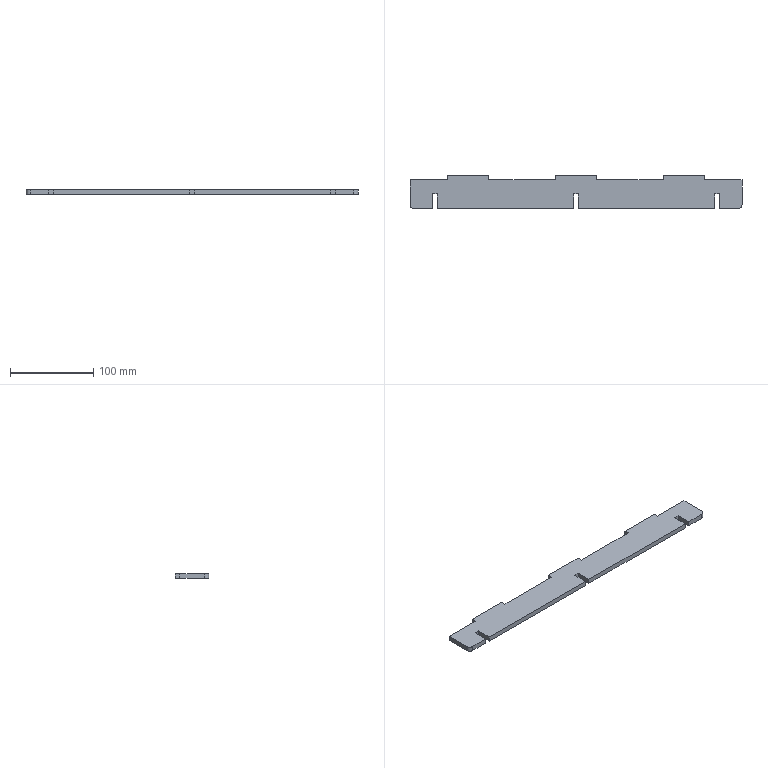Part | SolidWorks | features FlatPattern 1, SMBaseFlange 1, SheetMetal 1 | 1 solid | 32 faces | box 400 x 40.5 x 6 mm | volume 86942 mm3 | plane 30 | cylinder 2 | commonest cylinder face diameters 10 x2
STEP:
#1=CARTESIAN_POINT('',(-205.837,-343.504,0.));
#2=VERTEX_POINT('',#1);
#3=CARTESIAN_POINT('',(-205.837,-373.504,0.));
#4=VERTEX_POINT('',#3);
#5=CARTESIAN_POINT('',(-205.837,-343.504,0.));
#6=DIRECTION('',(0.,-1.,0.));
#7=VECTOR('',#6,1000.);
#8=LINE('',#5,#7);
#9=EDGE_CURVE('',#2,#4,#8,.T.);
#10=ORIENTED_EDGE('',*,*,#9,.F.);
#11=CARTESIAN_POINT('',(-205.837,-343.504,-6.));
#12=VERTEX_POINT('',#11);
#13=CARTESIAN_POINT('',(-205.837,-343.504,-6.));
#14=DIRECTION('',(0.,0.,1.));
#15=VECTOR('',#14,1000.);
#16=LINE('',#13,#15);
#17=EDGE_CURVE('',#12,#2,#16,.T.);
#18=ORIENTED_EDGE('',*,*,#17,.F.);
#19=CARTESIAN_POINT('',(-205.837,-373.504,-6.));
#20=VERTEX_POINT('',#19);
#21=CARTESIAN_POINT('',(-205.837,-343.504,-6.));
#22=DIRECTION('',(0.,-1.,0.));
#23=VECTOR('',#22,1000.);
#24=LINE('',#21,#23);
#25=EDGE_CURVE('',#12,#20,#24,.T.);
#26=ORIENTED_EDGE('',*,*,#25,.T.);
#27=CARTESIAN_POINT('',(-205.837,-373.504,-6.));
#28=DIRECTION('',(0.,0.,1.));
#29=VECTOR('',#28,1000.);
#30=LINE('',#27,#29);
#31=EDGE_CURVE('',#20,#4,#30,.T.);
#32=ORIENTED_EDGE('',*,*,#31,.T.);
#33=EDGE_LOOP('',(#10,#18,#26,#32));
#34=FACE_OUTER_BOUND('',#33,.T.);
#35=CARTESIAN_POINT('',(-205.837,-343.504,-6.));
#36=DIRECTION('',(-1.,0.,0.));
#37=DIRECTION('',(0.,0.,1.));
#38=AXIS2_PLACEMENT_3D('',#35,#36,#37);
#39=PLANE('',#38);
#40=ADVANCED_FACE('',(#34),#39,.T.);
#41=CARTESIAN_POINT('',(-160.837,-343.504,0.));
#42=VERTEX_POINT('',#41);
#43=CARTESIAN_POINT('',(-205.837,-343.504,0.));
#44=DIRECTION('',(-1.,0.,0.));
#45=VECTOR('',#44,1000.);
#46=LINE('',#43,#45);
#47=EDGE_CURVE('',#42,#2,#46,.T.);
#48=ORIENTED_EDGE('',*,*,#47,.F.);
#49=CARTESIAN_POINT('',(-160.837,-343.504,-6.));
#50=VERTEX_POINT('',#49);
#51=CARTESIAN_POINT('',(-160.837,-343.504,-6.));
#52=DIRECTION('',(0.,0.,1.));
#53=VECTOR('',#52,1000.);
#54=LINE('',#51,#53);
#55=EDGE_CURVE('',#50,#42,#54,.T.);
#56=ORIENTED_EDGE('',*,*,#55,.F.);
#57=CARTESIAN_POINT('',(-205.837,-343.504,-6.));
#58=DIRECTION('',(-1.,0.,0.));
#59=VECTOR('',#58,1000.);
#60=LINE('',#57,#59);
#61=EDGE_CURVE('',#50,#12,#60,.T.);
#62=ORIENTED_EDGE('',*,*,#61,.T.);
#63=ORIENTED_EDGE('',*,*,#17,.T.);
#64=EDGE_LOOP('',(#48,#56,#62,#63));
#65=FACE_OUTER_BOUND('',#64,.T.);
#66=CARTESIAN_POINT('',(-205.837,-343.504,-6.));
#67=DIRECTION('',(0.,1.,0.));
#68=DIRECTION('',(0.,0.,1.));
#69=AXIS2_PLACEMENT_3D('',#66,#67,#68);
#70=PLANE('',#69);
#71=ADVANCED_FACE('',(#65),#70,.T.);
#72=CARTESIAN_POINT('',(-160.837,-338.004,0.));
#73=VERTEX_POINT('',#72);
#74=CARTESIAN_POINT('',(-160.837,-343.504,0.));
#75=DIRECTION('',(0.,-1.,0.));
#76=VECTOR('',#75,1000.);
#77=LINE('',#74,#76);
#78=EDGE_CURVE('',#73,#42,#77,.T.);
#79=ORIENTED_EDGE('',*,*,#78,.F.);
#80=CARTESIAN_POINT('',(-160.837,-338.004,-6.));
#81=VERTEX_POINT('',#80);
#82=CARTESIAN_POINT('',(-160.837,-338.004,-6.));
#83=DIRECTION('',(0.,0.,1.));
#84=VECTOR('',#83,1000.);
#85=LINE('',#82,#84);
#86=EDGE_CURVE('',#81,#73,#85,.T.);
#87=ORIENTED_EDGE('',*,*,#86,.F.);
#88=CARTESIAN_POINT('',(-160.837,-343.504,-6.));
#89=DIRECTION('',(0.,-1.,0.));
#90=VECTOR('',#89,1000.);
#91=LINE('',#88,#90);
#92=EDGE_CURVE('',#81,#50,#91,.T.);
#93=ORIENTED_EDGE('',*,*,#92,.T.);
#94=ORIENTED_EDGE('',*,*,#55,.T.);
#95=EDGE_LOOP('',(#79,#87,#93,#94));
#96=FACE_OUTER_BOUND('',#95,.T.);
#97=CARTESIAN_POINT('',(-160.837,-343.504,-6.));
#98=DIRECTION('',(-1.,0.,0.));
#99=DIRECTION('',(0.,-1.,0.));
#100=AXIS2_PLACEMENT_3D('',#97,#98,#99);
#101=PLANE('',#100);
#102=ADVANCED_FACE('',(#96),#101,.T.);
#103=CARTESIAN_POINT('',(-110.837,-338.004,0.));
#104=VERTEX_POINT('',#103);
#105=CARTESIAN_POINT('',(-160.837,-338.004,0.));
#106=DIRECTION('',(-1.,0.,0.));
#107=VECTOR('',#106,1000.);
#108=LINE('',#105,#107);
#109=EDGE_CURVE('',#104,#73,#108,.T.);
#110=ORIENTED_EDGE('',*,*,#109,.F.);
#111=CARTESIAN_POINT('',(-110.837,-338.004,-6.));
#112=VERTEX_POINT('',#111);
#113=CARTESIAN_POINT('',(-110.837,-338.004,-6.));
#114=DIRECTION('',(0.,0.,1.));
#115=VECTOR('',#114,1000.);
#116=LINE('',#113,#115);
#117=EDGE_CURVE('',#112,#104,#116,.T.);
#118=ORIENTED_EDGE('',*,*,#117,.F.);
#119=CARTESIAN_POINT('',(-160.837,-338.004,-6.));
#120=DIRECTION('',(-1.,0.,0.));
#121=VECTOR('',#120,1000.);
#122=LINE('',#119,#121);
#123=EDGE_CURVE('',#112,#81,#122,.T.);
#124=ORIENTED_EDGE('',*,*,#123,.T.);
#125=ORIENTED_EDGE('',*,*,#86,.T.);
#126=EDGE_LOOP('',(#110,#118,#124,#125));
#127=FACE_OUTER_BOUND('',#126,.T.);
#128=CARTESIAN_POINT('',(-160.837,-338.004,-6.));
#129=DIRECTION('',(0.,1.,0.));
#130=DIRECTION('',(0.,0.,1.));
#131=AXIS2_PLACEMENT_3D('',#128,#129,#130);
#132=PLANE('',#131);
#133=ADVANCED_FACE('',(#127),#132,.T.);
#134=CARTESIAN_POINT('',(-110.837,-343.504,0.));
#135=VERTEX_POINT('',#134);
#136=CARTESIAN_POINT('',(-110.837,-338.004,0.));
#137=DIRECTION('',(0.,1.,0.));
#138=VECTOR('',#137,1000.);
#139=LINE('',#136,#138);
#140=EDGE_CURVE('',#135,#104,#139,.T.);
#141=ORIENTED_EDGE('',*,*,#140,.F.);
#142=CARTESIAN_POINT('',(-110.837,-343.504,-6.));
#143=VERTEX_POINT('',#142);
#144=CARTESIAN_POINT('',(-110.837,-343.504,-6.));
#145=DIRECTION('',(0.,0.,1.));
#146=VECTOR('',#145,1000.);
#147=LINE('',#144,#146);
#148=EDGE_CURVE('',#143,#135,#147,.T.);
#149=ORIENTED_EDGE('',*,*,#148,.F.);
#150=CARTESIAN_POINT('',(-110.837,-338.004,-6.));
#151=DIRECTION('',(0.,1.,0.));
#152=VECTOR('',#151,1000.);
#153=LINE('',#150,#152);
#154=EDGE_CURVE('',#143,#112,#153,.T.);
#155=ORIENTED_EDGE('',*,*,#154,.T.);
#156=ORIENTED_EDGE('',*,*,#117,.T.);
#157=EDGE_LOOP('',(#141,#149,#155,#156));
#158=FACE_OUTER_BOUND('',#157,.T.);
#159=CARTESIAN_POINT('',(-110.837,-338.004,-6.));
#160=DIRECTION('',(1.,0.,0.));
#161=DIRECTION('',(0.,1.,0.));
#162=AXIS2_PLACEMENT_3D('',#159,#160,#161);
#163=PLANE('',#162);
#164=ADVANCED_FACE('',(#158),#163,.T.);
#165=CARTESIAN_POINT('',(-30.837,-343.504,0.));
#166=VERTEX_POINT('',#165);
#167=CARTESIAN_POINT('',(-110.837,-343.504,0.));
#168=DIRECTION('',(-1.,0.,0.));
#169=VECTOR('',#168,1000.);
#170=LINE('',#167,#169);
#171=EDGE_CURVE('',#166,#135,#170,.T.);
#172=ORIENTED_EDGE('',*,*,#171,.F.);
#173=CARTESIAN_POINT('',(-30.837,-343.504,-6.));
#174=VERTEX_POINT('',#173);
#175=CARTESIAN_POINT('',(-30.837,-343.504,-6.));
#176=DIRECTION('',(0.,0.,1.));
#177=VECTOR('',#176,1000.);
#178=LINE('',#175,#177);
#179=EDGE_CURVE('',#174,#166,#178,.T.);
#180=ORIENTED_EDGE('',*,*,#179,.F.);
#181=CARTESIAN_POINT('',(-110.837,-343.504,-6.));
#182=DIRECTION('',(-1.,0.,0.));
#183=VECTOR('',#182,1000.);
#184=LINE('',#181,#183);
#185=EDGE_CURVE('',#174,#143,#184,.T.);
#186=ORIENTED_EDGE('',*,*,#185,.T.);
#187=ORIENTED_EDGE('',*,*,#148,.T.);
#188=EDGE_LOOP('',(#172,#180,#186,#187));
#189=FACE_OUTER_BOUND('',#188,.T.);
#190=CARTESIAN_POINT('',(-110.837,-343.504,-6.));
#191=DIRECTION('',(0.,1.,0.));
#192=DIRECTION('',(0.,0.,1.));
#193=AXIS2_PLACEMENT_3D('',#190,#191,#192);
#194=PLANE('',#193);
#195=ADVANCED_FACE('',(#189),#194,.T.);
#196=CARTESIAN_POINT('',(-30.837,-338.004,0.));
#197=VERTEX_POINT('',#196);
#198=CARTESIAN_POINT('',(-30.837,-338.004,0.));
#199=DIRECTION('',(0.,-1.,0.));
#200=VECTOR('',#199,1000.);
#201=LINE('',#198,#200);
#202=EDGE_CURVE('',#197,#166,#201,.T.);
#203=ORIENTED_EDGE('',*,*,#202,.F.);
#204=CARTESIAN_POINT('',(-30.837,-338.004,-6.));
#205=VERTEX_POINT('',#204);
#206=CARTESIAN_POINT('',(-30.837,-338.004,-6.));
#207=DIRECTION('',(0.,0.,1.));
#208=VECTOR('',#207,1000.);
#209=LINE('',#206,#208);
#210=EDGE_CURVE('',#205,#197,#209,.T.);
#211=ORIENTED_EDGE('',*,*,#210,.F.);
#212=CARTESIAN_POINT('',(-30.837,-338.004,-6.));
#213=DIRECTION('',(0.,-1.,0.));
#214=VECTOR('',#213,1000.);
#215=LINE('',#212,#214);
#216=EDGE_CURVE('',#205,#174,#215,.T.);
#217=ORIENTED_EDGE('',*,*,#216,.T.);
#218=ORIENTED_EDGE('',*,*,#179,.T.);
#219=EDGE_LOOP('',(#203,#211,#217,#218));
#220=FACE_OUTER_BOUND('',#219,.T.);
#221=CARTESIAN_POINT('',(-30.837,-338.004,-6.));
#222=DIRECTION('',(-1.,0.,0.));
#223=DIRECTION('',(0.,-1.,0.));
#224=AXIS2_PLACEMENT_3D('',#221,#222,#223);
#225=PLANE('',#224);
#226=ADVANCED_FACE('',(#220),#225,.T.);
#227=CARTESIAN_POINT('',(19.163,-338.004,0.));
#228=VERTEX_POINT('',#227);
#229=CARTESIAN_POINT('',(19.163,-338.004,0.));
#230=DIRECTION('',(-1.,0.,0.));
#231=VECTOR('',#230,1000.);
#232=LINE('',#229,#231);
#233=EDGE_CURVE('',#228,#197,#232,.T.);
#234=ORIENTED_EDGE('',*,*,#233,.F.);
#235=CARTESIAN_POINT('',(19.163,-338.004,-6.));
#236=VERTEX_POINT('',#235);
#237=CARTESIAN_POINT('',(19.163,-338.004,-6.));
#238=DIRECTION('',(0.,0.,1.));
#239=VECTOR('',#238,1000.);
#240=LINE('',#237,#239);
#241=EDGE_CURVE('',#236,#228,#240,.T.);
#242=ORIENTED_EDGE('',*,*,#241,.F.);
#243=CARTESIAN_POINT('',(19.163,-338.004,-6.));
#244=DIRECTION('',(-1.,0.,0.));
#245=VECTOR('',#244,1000.);
#246=LINE('',#243,#245);
#247=EDGE_CURVE('',#236,#205,#246,.T.);
#248=ORIENTED_EDGE('',*,*,#247,.T.);
#249=ORIENTED_EDGE('',*,*,#210,.T.);
#250=EDGE_LOOP('',(#234,#242,#248,#249));
#251=FACE_OUTER_BOUND('',#250,.T.);
#252=CARTESIAN_POINT('',(19.163,-338.004,-6.));
#253=DIRECTION('',(0.,1.,0.));
#254=DIRECTION('',(0.,0.,1.));
#255=AXIS2_PLACEMENT_3D('',#252,#253,#254);
#256=PLANE('',#255);
#257=ADVANCED_FACE('',(#251),#256,.T.);
#258=CARTESIAN_POINT('',(19.163,-343.504,0.));
#259=VERTEX_POINT('',#258);
#260=CARTESIAN_POINT('',(19.163,-343.504,0.));
#261=DIRECTION('',(0.,1.,0.));
#262=VECTOR('',#261,1000.);
#263=LINE('',#260,#262);
#264=EDGE_CURVE('',#259,#228,#263,.T.);
#265=ORIENTED_EDGE('',*,*,#264,.F.);
#266=CARTESIAN_POINT('',(19.163,-343.504,-6.));
#267=VERTEX_POINT('',#266);
#268=CARTESIAN_POINT('',(19.163,-343.504,-6.));
#269=DIRECTION('',(0.,0.,1.));
#270=VECTOR('',#269,1000.);
#271=LINE('',#268,#270);
#272=EDGE_CURVE('',#267,#259,#271,.T.);
#273=ORIENTED_EDGE('',*,*,#272,.F.);
#274=CARTESIAN_POINT('',(19.163,-343.504,-6.));
#275=DIRECTION('',(0.,1.,0.));
#276=VECTOR('',#275,1000.);
#277=LINE('',#274,#276);
#278=EDGE_CURVE('',#267,#236,#277,.T.);
#279=ORIENTED_EDGE('',*,*,#278,.T.);
#280=ORIENTED_EDGE('',*,*,#241,.T.);
#281=EDGE_LOOP('',(#265,#273,#279,#280));
#282=FACE_OUTER_BOUND('',#281,.T.);
#283=CARTESIAN_POINT('',(19.163,-343.504,-6.));
#284=DIRECTION('',(1.,0.,0.));
#285=DIRECTION('',(0.,1.,0.));
#286=AXIS2_PLACEMENT_3D('',#283,#284,#285);
#287=PLANE('',#286);
#288=ADVANCED_FACE('',(#282),#287,.T.);
#289=CARTESIAN_POINT('',(99.163,-343.504,0.));
#290=VERTEX_POINT('',#289);
#291=CARTESIAN_POINT('',(19.163,-343.504,0.));
#292=DIRECTION('',(-1.,0.,0.));
#293=VECTOR('',#292,1000.);
#294=LINE('',#291,#293);
#295=EDGE_CURVE('',#290,#259,#294,.T.);
#296=ORIENTED_EDGE('',*,*,#295,.F.);
#297=CARTESIAN_POINT('',(99.163,-343.504,-6.));
#298=VERTEX_POINT('',#297);
#299=CARTESIAN_POINT('',(99.163,-343.504,-6.));
#300=DIRECTION('',(0.,0.,1.));
#301=VECTOR('',#300,1000.);
#302=LINE('',#299,#301);
#303=EDGE_CURVE('',#298,#290,#302,.T.);
#304=ORIENTED_EDGE('',*,*,#303,.F.);
#305=CARTESIAN_POINT('',(19.163,-343.504,-6.));
#306=DIRECTION('',(-1.,0.,0.));
#307=VECTOR('',#306,1000.);
#308=LINE('',#305,#307);
#309=EDGE_CURVE('',#298,#267,#308,.T.);
#310=ORIENTED_EDGE('',*,*,#309,.T.);
#311=ORIENTED_EDGE('',*,*,#272,.T.);
#312=EDGE_LOOP('',(#296,#304,#310,#311));
#313=FACE_OUTER_BOUND('',#312,.T.);
#314=CARTESIAN_POINT('',(19.163,-343.504,-6.));
#315=DIRECTION('',(0.,1.,0.));
#316=DIRECTION('',(0.,0.,1.));
#317=AXIS2_PLACEMENT_3D('',#314,#315,#316);
#318=PLANE('',#317);
#319=ADVANCED_FACE('',(#313),#318,.T.);
#320=CARTESIAN_POINT('',(99.163,-338.004,0.));
#321=VERTEX_POINT('',#320);
#322=CARTESIAN_POINT('',(99.163,-338.004,0.));
#323=DIRECTION('',(0.,-1.,0.));
#324=VECTOR('',#323,1000.);
#325=LINE('',#322,#324);
#326=EDGE_CURVE('',#321,#290,#325,.T.);
#327=ORIENTED_EDGE('',*,*,#326,.F.);
#328=CARTESIAN_POINT('',(99.163,-338.004,-6.));
#329=VERTEX_POINT('',#328);
#330=CARTESIAN_POINT('',(99.163,-338.004,-6.));
#331=DIRECTION('',(0.,0.,1.));
#332=VECTOR('',#331,1000.);
#333=LINE('',#330,#332);
#334=EDGE_CURVE('',#329,#321,#333,.T.);
#335=ORIENTED_EDGE('',*,*,#334,.F.);
#336=CARTESIAN_POINT('',(99.163,-338.004,-6.));
#337=DIRECTION('',(0.,-1.,0.));
#338=VECTOR('',#337,1000.);
#339=LINE('',#336,#338);
#340=EDGE_CURVE('',#329,#298,#339,.T.);
#341=ORIENTED_EDGE('',*,*,#340,.T.);
#342=ORIENTED_EDGE('',*,*,#303,.T.);
#343=EDGE_LOOP('',(#327,#335,#341,#342));
#344=FACE_OUTER_BOUND('',#343,.T.);
#345=CARTESIAN_POINT('',(99.163,-338.004,-6.));
#346=DIRECTION('',(-1.,0.,0.));
#347=DIRECTION('',(0.,0.,1.));
#348=AXIS2_PLACEMENT_3D('',#345,#346,#347);
#349=PLANE('',#348);
#350=ADVANCED_FACE('',(#344),#349,.T.);
#351=CARTESIAN_POINT('',(149.163,-338.004,0.));
#352=VERTEX_POINT('',#351);
#353=CARTESIAN_POINT('',(149.163,-338.004,0.));
#354=DIRECTION('',(-1.,0.,0.));
#355=VECTOR('',#354,1000.);
#356=LINE('',#353,#355);
#357=EDGE_CURVE('',#352,#321,#356,.T.);
#358=ORIENTED_EDGE('',*,*,#357,.F.);
#359=CARTESIAN_POINT('',(149.163,-338.004,-6.));
#360=VERTEX_POINT('',#359);
#361=CARTESIAN_POINT('',(149.163,-338.004,-6.));
#362=DIRECTION('',(0.,0.,1.));
#363=VECTOR('',#362,1000.);
#364=LINE('',#361,#363);
#365=EDGE_CURVE('',#360,#352,#364,.T.);
#366=ORIENTED_EDGE('',*,*,#365,.F.);
#367=CARTESIAN_POINT('',(149.163,-338.004,-6.));
#368=DIRECTION('',(-1.,0.,0.));
#369=VECTOR('',#368,1000.);
#370=LINE('',#367,#369);
#371=EDGE_CURVE('',#360,#329,#370,.T.);
#372=ORIENTED_EDGE('',*,*,#371,.T.);
#373=ORIENTED_EDGE('',*,*,#334,.T.);
#374=EDGE_LOOP('',(#358,#366,#372,#373));
#375=FACE_OUTER_BOUND('',#374,.T.);
#376=CARTESIAN_POINT('',(149.163,-338.004,-6.));
#377=DIRECTION('',(0.,1.,0.));
#378=DIRECTION('',(0.,0.,1.));
#379=AXIS2_PLACEMENT_3D('',#376,#377,#378);
#380=PLANE('',#379);
#381=ADVANCED_FACE('',(#375),#380,.T.);
#382=CARTESIAN_POINT('',(149.163,-343.504,0.));
#383=VERTEX_POINT('',#382);
#384=CARTESIAN_POINT('',(149.163,-343.504,0.));
#385=DIRECTION('',(0.,1.,0.));
#386=VECTOR('',#385,1000.);
#387=LINE('',#384,#386);
#388=EDGE_CURVE('',#383,#352,#387,.T.);
#389=ORIENTED_EDGE('',*,*,#388,.F.);
#390=CARTESIAN_POINT('',(149.163,-343.504,-6.));
#391=VERTEX_POINT('',#390);
#392=CARTESIAN_POINT('',(149.163,-343.504,-6.));
#393=DIRECTION('',(0.,0.,1.));
#394=VECTOR('',#393,1000.);
#395=LINE('',#392,#394);
#396=EDGE_CURVE('',#391,#383,#395,.T.);
#397=ORIENTED_EDGE('',*,*,#396,.F.);
#398=CARTESIAN_POINT('',(149.163,-343.504,-6.));
#399=DIRECTION('',(0.,1.,0.));
#400=VECTOR('',#399,1000.);
#401=LINE('',#398,#400);
#402=EDGE_CURVE('',#391,#360,#401,.T.);
#403=ORIENTED_EDGE('',*,*,#402,.T.);
#404=ORIENTED_EDGE('',*,*,#365,.T.);
#405=EDGE_LOOP('',(#389,#397,#403,#404));
#406=FACE_OUTER_BOUND('',#405,.T.);
#407=CARTESIAN_POINT('',(149.163,-343.504,-6.));
#408=DIRECTION('',(1.,0.,0.));
#409=DIRECTION('',(0.,0.,-1.));
#410=AXIS2_PLACEMENT_3D('',#407,#408,#409);
#411=PLANE('',#410);
#412=ADVANCED_FACE('',(#406),#411,.T.);
#413=CARTESIAN_POINT('',(194.163,-343.504,0.));
#414=VERTEX_POINT('',#413);
#415=CARTESIAN_POINT('',(149.163,-343.504,0.));
#416=DIRECTION('',(-1.,0.,0.));
#417=VECTOR('',#416,1000.);
#418=LINE('',#415,#417);
#419=EDGE_CURVE('',#414,#383,#418,.T.);
#420=ORIENTED_EDGE('',*,*,#419,.F.);
#421=CARTESIAN_POINT('',(194.163,-343.504,-6.));
#422=VERTEX_POINT('',#421);
#423=CARTESIAN_POINT('',(194.163,-343.504,-6.));
#424=DIRECTION('',(0.,0.,1.));
#425=VECTOR('',#424,1000.);
#426=LINE('',#423,#425);
#427=EDGE_CURVE('',#422,#414,#426,.T.);
#428=ORIENTED_EDGE('',*,*,#427,.F.);
#429=CARTESIAN_POINT('',(149.163,-343.504,-6.));
#430=DIRECTION('',(-1.,0.,0.));
#431=VECTOR('',#430,1000.);
#432=LINE('',#429,#431);
#433=EDGE_CURVE('',#422,#391,#432,.T.);
#434=ORIENTED_EDGE('',*,*,#433,.T.);
#435=ORIENTED_EDGE('',*,*,#396,.T.);
#436=EDGE_LOOP('',(#420,#428,#434,#435));
#437=FACE_OUTER_BOUND('',#436,.T.);
#438=CARTESIAN_POINT('',(149.163,-343.504,-6.));
#439=DIRECTION('',(0.,1.,0.));
#440=DIRECTION('',(0.,0.,1.));
#441=AXIS2_PLACEMENT_3D('',#438,#439,#440);
#442=PLANE('',#441);
#443=ADVANCED_FACE('',(#437),#442,.T.);
#444=CARTESIAN_POINT('',(194.163,-373.504,0.));
#445=VERTEX_POINT('',#444);
#446=CARTESIAN_POINT('',(194.163,-343.504,0.));
#447=DIRECTION('',(0.,1.,0.));
#448=VECTOR('',#447,1000.);
#449=LINE('',#446,#448);
#450=EDGE_CURVE('',#445,#414,#449,.T.);
#451=ORIENTED_EDGE('',*,*,#450,.F.);
#452=CARTESIAN_POINT('',(194.163,-373.504,-6.));
#453=VERTEX_POINT('',#452);
#454=CARTESIAN_POINT('',(194.163,-373.504,-6.));
#455=DIRECTION('',(0.,0.,1.));
#456=VECTOR('',#455,1000.);
#457=LINE('',#454,#456);
#458=EDGE_CURVE('',#453,#445,#457,.T.);
#459=ORIENTED_EDGE('',*,*,#458,.F.);
#460=CARTESIAN_POINT('',(194.163,-343.504,-6.));
#461=DIRECTION('',(0.,1.,0.));
#462=VECTOR('',#461,1000.);
#463=LINE('',#460,#462);
#464=EDGE_CURVE('',#453,#422,#463,.T.);
#465=ORIENTED_EDGE('',*,*,#464,.T.);
#466=ORIENTED_EDGE('',*,*,#427,.T.);
#467=EDGE_LOOP('',(#451,#459,#465,#466));
#468=FACE_OUTER_BOUND('',#467,.T.);
#469=CARTESIAN_POINT('',(194.163,-343.504,-6.));
#470=DIRECTION('',(1.,0.,0.));
#471=DIRECTION('',(0.,0.,-1.));
#472=AXIS2_PLACEMENT_3D('',#469,#470,#471);
#473=PLANE('',#472);
#474=ADVANCED_FACE('',(#468),#473,.T.);
#475=CARTESIAN_POINT('',(189.163,-378.504,0.));
#476=VERTEX_POINT('',#475);
#477=CARTESIAN_POINT('',(189.163,-373.504,0.));
#478=DIRECTION('',(0.,0.,1.));
#479=DIRECTION('',(1.,0.,0.));
#480=AXIS2_PLACEMENT_3D('',#477,#478,#479);
#481=CIRCLE('',#480,5.);
#482=EDGE_CURVE('',#476,#445,#481,.T.);
#483=ORIENTED_EDGE('',*,*,#482,.F.);
#484=CARTESIAN_POINT('',(189.163,-378.504,-6.));
#485=VERTEX_POINT('',#484);
#486=CARTESIAN_POINT('',(189.163,-378.504,-6.));
#487=DIRECTION('',(0.,0.,1.));
#488=VECTOR('',#487,1000.);
#489=LINE('',#486,#488);
#490=EDGE_CURVE('',#485,#476,#489,.T.);
#491=ORIENTED_EDGE('',*,*,#490,.F.);
#492=CARTESIAN_POINT('',(189.163,-373.504,-6.));
#493=DIRECTION('',(0.,0.,1.));
#494=DIRECTION('',(1.,0.,0.));
#495=AXIS2_PLACEMENT_3D('',#492,#493,#494);
#496=CIRCLE('',#495,5.);
#497=EDGE_CURVE('',#485,#453,#496,.T.);
#498=ORIENTED_EDGE('',*,*,#497,.T.);
#499=ORIENTED_EDGE('',*,*,#458,.T.);
#500=EDGE_LOOP('',(#483,#491,#498,#499));
#501=FACE_OUTER_BOUND('',#500,.T.);
#502=CARTESIAN_POINT('',(189.163,-373.504,-6.));
#503=DIRECTION('',(0.,0.,1.));
#504=DIRECTION('',(1.,0.,0.));
#505=AXIS2_PLACEMENT_3D('',#502,#503,#504);
#506=CYLINDRICAL_SURFACE('',#505,5.);
#507=ADVANCED_FACE('',(#501),#506,.T.);
#508=CARTESIAN_POINT('',(167.163,-378.504,0.));
#509=VERTEX_POINT('',#508);
#510=CARTESIAN_POINT('',(167.163,-378.504,0.));
#511=DIRECTION('',(1.,0.,0.));
#512=VECTOR('',#511,1000.);
#513=LINE('',#510,#512);
#514=EDGE_CURVE('',#509,#476,#513,.T.);
#515=ORIENTED_EDGE('',*,*,#514,.F.);
#516=CARTESIAN_POINT('',(167.163,-378.504,-6.));
#517=VERTEX_POINT('',#516);
#518=CARTESIAN_POINT('',(167.163,-378.504,-6.));
#519=DIRECTION('',(0.,0.,1.));
#520=VECTOR('',#519,1000.);
#521=LINE('',#518,#520);
#522=EDGE_CURVE('',#517,#509,#521,.T.);
#523=ORIENTED_EDGE('',*,*,#522,.F.);
#524=CARTESIAN_POINT('',(167.163,-378.504,-6.));
#525=DIRECTION('',(1.,0.,0.));
#526=VECTOR('',#525,1000.);
#527=LINE('',#524,#526);
#528=EDGE_CURVE('',#517,#485,#527,.T.);
#529=ORIENTED_EDGE('',*,*,#528,.T.);
#530=ORIENTED_EDGE('',*,*,#490,.T.);
#531=EDGE_LOOP('',(#515,#523,#529,#530));
#532=FACE_OUTER_BOUND('',#531,.T.);
#533=CARTESIAN_POINT('',(167.163,-378.504,-6.));
#534=DIRECTION('',(0.,-1.,0.));
#535=DIRECTION('',(0.,0.,-1.));
#536=AXIS2_PLACEMENT_3D('',#533,#534,#535);
#537=PLANE('',#536);
#538=ADVANCED_FACE('',(#532),#537,.T.);
#539=CARTESIAN_POINT('',(167.163,-360.504,0.));
#540=VERTEX_POINT('',#539);
#541=CARTESIAN_POINT('',(167.163,-360.504,0.));
#542=DIRECTION('',(0.,-1.,0.));
#543=VECTOR('',#542,1000.);
#544=LINE('',#541,#543);
#545=EDGE_CURVE('',#540,#509,#544,.T.);
#546=ORIENTED_EDGE('',*,*,#545,.F.);
#547=CARTESIAN_POINT('',(167.163,-360.504,-6.));
#548=VERTEX_POINT('',#547);
#549=CARTESIAN_POINT('',(167.163,-360.504,-6.));
#550=DIRECTION('',(0.,0.,1.));
#551=VECTOR('',#550,1000.);
#552=LINE('',#549,#551);
#553=EDGE_CURVE('',#548,#540,#552,.T.);
#554=ORIENTED_EDGE('',*,*,#553,.F.);
#555=CARTESIAN_POINT('',(167.163,-360.504,-6.));
#556=DIRECTION('',(0.,-1.,0.));
#557=VECTOR('',#556,1000.);
#558=LINE('',#555,#557);
#559=EDGE_CURVE('',#548,#517,#558,.T.);
#560=ORIENTED_EDGE('',*,*,#559,.T.);
#561=ORIENTED_EDGE('',*,*,#522,.T.);
#562=EDGE_LOOP('',(#546,#554,#560,#561));
#563=FACE_OUTER_BOUND('',#562,.T.);
#564=CARTESIAN_POINT('',(167.163,-360.504,-6.));
#565=DIRECTION('',(-1.,0.,0.));
#566=DIRECTION('',(0.,0.,1.));
#567=AXIS2_PLACEMENT_3D('',#564,#565,#566);
#568=PLANE('',#567);
#569=ADVANCED_FACE('',(#563),#568,.T.);
#570=CARTESIAN_POINT('',(161.163,-360.504,0.));
#571=VERTEX_POINT('',#570);
#572=CARTESIAN_POINT('',(161.163,-360.504,0.));
#573=DIRECTION('',(1.,0.,0.));
#574=VECTOR('',#573,1000.);
#575=LINE('',#572,#574);
#576=EDGE_CURVE('',#571,#540,#575,.T.);
#577=ORIENTED_EDGE('',*,*,#576,.F.);
#578=CARTESIAN_POINT('',(161.163,-360.504,-6.));
#579=VERTEX_POINT('',#578);
#580=CARTESIAN_POINT('',(161.163,-360.504,-6.));
#581=DIRECTION('',(0.,0.,1.));
#582=VECTOR('',#581,1000.);
#583=LINE('',#580,#582);
#584=EDGE_CURVE('',#579,#571,#583,.T.);
#585=ORIENTED_EDGE('',*,*,#584,.F.);
#586=CARTESIAN_POINT('',(161.163,-360.504,-6.));
#587=DIRECTION('',(1.,0.,0.));
#588=VECTOR('',#587,1000.);
#589=LINE('',#586,#588);
#590=EDGE_CURVE('',#579,#548,#589,.T.);
#591=ORIENTED_EDGE('',*,*,#590,.T.);
#592=ORIENTED_EDGE('',*,*,#553,.T.);
#593=EDGE_LOOP('',(#577,#585,#591,#592));
#594=FACE_OUTER_BOUND('',#593,.T.);
#595=CARTESIAN_POINT('',(161.163,-360.504,-6.));
#596=DIRECTION('',(0.,-1.,0.));
#597=DIRECTION('',(0.,0.,-1.));
#598=AXIS2_PLACEMENT_3D('',#595,#596,#597);
#599=PLANE('',#598);
#600=ADVANCED_FACE('',(#594),#599,.T.);
#601=CARTESIAN_POINT('',(161.163,-378.504,0.));
#602=VERTEX_POINT('',#601);
#603=CARTESIAN_POINT('',(161.163,-378.504,0.));
#604=DIRECTION('',(0.,1.,0.));
#605=VECTOR('',#604,1000.);
#606=LINE('',#603,#605);
#607=EDGE_CURVE('',#602,#571,#606,.T.);
#608=ORIENTED_EDGE('',*,*,#607,.F.);
#609=CARTESIAN_POINT('',(161.163,-378.504,-6.));
#610=VERTEX_POINT('',#609);
#611=CARTESIAN_POINT('',(161.163,-378.504,-6.));
#612=DIRECTION('',(0.,0.,1.));
#613=VECTOR('',#612,1000.);
#614=LINE('',#611,#613);
#615=EDGE_CURVE('',#610,#602,#614,.T.);
#616=ORIENTED_EDGE('',*,*,#615,.F.);
#617=CARTESIAN_POINT('',(161.163,-378.504,-6.));
#618=DIRECTION('',(0.,1.,0.));
#619=VECTOR('',#618,1000.);
#620=LINE('',#617,#619);
#621=EDGE_CURVE('',#610,#579,#620,.T.);
#622=ORIENTED_EDGE('',*,*,#621,.T.);
#623=ORIENTED_EDGE('',*,*,#584,.T.);
#624=EDGE_LOOP('',(#608,#616,#622,#623));
#625=FACE_OUTER_BOUND('',#624,.T.);
#626=CARTESIAN_POINT('',(161.163,-378.504,-6.));
#627=DIRECTION('',(1.,0.,0.));
#628=DIRECTION('',(0.,0.,-1.));
#629=AXIS2_PLACEMENT_3D('',#626,#627,#628);
#630=PLANE('',#629);
#631=ADVANCED_FACE('',(#625),#630,.T.);
#632=CARTESIAN_POINT('',(-2.837,-378.504,0.));
#633=VERTEX_POINT('',#632);
#634=CARTESIAN_POINT('',(-2.837,-378.504,0.));
#635=DIRECTION('',(1.,0.,0.));
#636=VECTOR('',#635,1000.);
#637=LINE('',#634,#636);
#638=EDGE_CURVE('',#633,#602,#637,.T.);
#639=ORIENTED_EDGE('',*,*,#638,.F.);
#640=CARTESIAN_POINT('',(-2.837,-378.504,-6.));
#641=VERTEX_POINT('',#640);
#642=CARTESIAN_POINT('',(-2.837,-378.504,-6.));
#643=DIRECTION('',(0.,0.,1.));
#644=VECTOR('',#643,1000.);
#645=LINE('',#642,#644);
#646=EDGE_CURVE('',#641,#633,#645,.T.);
#647=ORIENTED_EDGE('',*,*,#646,.F.);
#648=CARTESIAN_POINT('',(-2.837,-378.504,-6.));
#649=DIRECTION('',(1.,0.,0.));
#650=VECTOR('',#649,1000.);
#651=LINE('',#648,#650);
#652=EDGE_CURVE('',#641,#610,#651,.T.);
#653=ORIENTED_EDGE('',*,*,#652,.T.);
#654=ORIENTED_EDGE('',*,*,#615,.T.);
#655=EDGE_LOOP('',(#639,#647,#653,#654));
#656=FACE_OUTER_BOUND('',#655,.T.);
#657=CARTESIAN_POINT('',(-2.837,-378.504,-6.));
#658=DIRECTION('',(0.,-1.,0.));
#659=DIRECTION('',(0.,0.,-1.));
#660=AXIS2_PLACEMENT_3D('',#657,#658,#659);
#661=PLANE('',#660);
#662=ADVANCED_FACE('',(#656),#661,.T.);
#663=CARTESIAN_POINT('',(-2.837,-360.504,0.));
#664=VERTEX_POINT('',#663);
#665=CARTESIAN_POINT('',(-2.837,-360.504,0.));
#666=DIRECTION('',(0.,-1.,0.));
#667=VECTOR('',#666,1000.);
#668=LINE('',#665,#667);
#669=EDGE_CURVE('',#664,#633,#668,.T.);
#670=ORIENTED_EDGE('',*,*,#669,.F.);
#671=CARTESIAN_POINT('',(-2.837,-360.504,-6.));
#672=VERTEX_POINT('',#671);
#673=CARTESIAN_POINT('',(-2.837,-360.504,-6.));
#674=DIRECTION('',(0.,0.,1.));
#675=VECTOR('',#674,1000.);
#676=LINE('',#673,#675);
#677=EDGE_CURVE('',#672,#664,#676,.T.);
#678=ORIENTED_EDGE('',*,*,#677,.F.);
#679=CARTESIAN_POINT('',(-2.837,-360.504,-6.));
#680=DIRECTION('',(0.,-1.,0.));
#681=VECTOR('',#680,1000.);
#682=LINE('',#679,#681);
#683=EDGE_CURVE('',#672,#641,#682,.T.);
#684=ORIENTED_EDGE('',*,*,#683,.T.);
#685=ORIENTED_EDGE('',*,*,#646,.T.);
#686=EDGE_LOOP('',(#670,#678,#684,#685));
#687=FACE_OUTER_BOUND('',#686,.T.);
#688=CARTESIAN_POINT('',(-2.837,-360.504,-6.));
#689=DIRECTION('',(-1.,0.,0.));
#690=DIRECTION('',(0.,0.,1.));
#691=AXIS2_PLACEMENT_3D('',#688,#689,#690);
#692=PLANE('',#691);
#693=ADVANCED_FACE('',(#687),#692,.T.);
#694=CARTESIAN_POINT('',(-8.837,-360.504,0.));
#695=VERTEX_POINT('',#694);
#696=CARTESIAN_POINT('',(-8.837,-360.504,0.));
#697=DIRECTION('',(1.,0.,0.));
#698=VECTOR('',#697,1000.);
#699=LINE('',#696,#698);
#700=EDGE_CURVE('',#695,#664,#699,.T.);
#701=ORIENTED_EDGE('',*,*,#700,.F.);
#702=CARTESIAN_POINT('',(-8.837,-360.504,-6.));
#703=VERTEX_POINT('',#702);
#704=CARTESIAN_POINT('',(-8.837,-360.504,-6.));
#705=DIRECTION('',(0.,0.,1.));
#706=VECTOR('',#705,1000.);
#707=LINE('',#704,#706);
#708=EDGE_CURVE('',#703,#695,#707,.T.);
#709=ORIENTED_EDGE('',*,*,#708,.F.);
#710=CARTESIAN_POINT('',(-8.837,-360.504,-6.));
#711=DIRECTION('',(1.,0.,0.));
#712=VECTOR('',#711,1000.);
#713=LINE('',#710,#712);
#714=EDGE_CURVE('',#703,#672,#713,.T.);
#715=ORIENTED_EDGE('',*,*,#714,.T.);
#716=ORIENTED_EDGE('',*,*,#677,.T.);
#717=EDGE_LOOP('',(#701,#709,#715,#716));
#718=FACE_OUTER_BOUND('',#717,.T.);
#719=CARTESIAN_POINT('',(-8.837,-360.504,-6.));
#720=DIRECTION('',(0.,-1.,0.));
#721=DIRECTION('',(0.,0.,-1.));
#722=AXIS2_PLACEMENT_3D('',#719,#720,#721);
#723=PLANE('',#722);
#724=ADVANCED_FACE('',(#718),#723,.T.);
#725=CARTESIAN_POINT('',(-8.837,-378.504,0.));
#726=VERTEX_POINT('',#725);
#727=CARTESIAN_POINT('',(-8.837,-378.504,0.));
#728=DIRECTION('',(0.,1.,0.));
#729=VECTOR('',#728,1000.);
#730=LINE('',#727,#729);
#731=EDGE_CURVE('',#726,#695,#730,.T.);
#732=ORIENTED_EDGE('',*,*,#731,.F.);
#733=CARTESIAN_POINT('',(-8.837,-378.504,-6.));
#734=VERTEX_POINT('',#733);
#735=CARTESIAN_POINT('',(-8.837,-378.504,-6.));
#736=DIRECTION('',(0.,0.,1.));
#737=VECTOR('',#736,1000.);
#738=LINE('',#735,#737);
#739=EDGE_CURVE('',#734,#726,#738,.T.);
#740=ORIENTED_EDGE('',*,*,#739,.F.);
#741=CARTESIAN_POINT('',(-8.837,-378.504,-6.));
#742=DIRECTION('',(0.,1.,0.));
#743=VECTOR('',#742,1000.);
#744=LINE('',#741,#743);
#745=EDGE_CURVE('',#734,#703,#744,.T.);
#746=ORIENTED_EDGE('',*,*,#745,.T.);
#747=ORIENTED_EDGE('',*,*,#708,.T.);
#748=EDGE_LOOP('',(#732,#740,#746,#747));
#749=FACE_OUTER_BOUND('',#748,.T.);
#750=CARTESIAN_POINT('',(-8.837,-378.504,-6.));
#751=DIRECTION('',(1.,0.,0.));
#752=DIRECTION('',(0.,1.,0.));
#753=AXIS2_PLACEMENT_3D('',#750,#751,#752);
#754=PLANE('',#753);
#755=ADVANCED_FACE('',(#749),#754,.T.);
#756=CARTESIAN_POINT('',(-172.837,-378.504,0.));
#757=VERTEX_POINT('',#756);
#758=CARTESIAN_POINT('',(-172.837,-378.504,0.));
#759=DIRECTION('',(1.,0.,0.));
#760=VECTOR('',#759,1000.);
#761=LINE('',#758,#760);
#762=EDGE_CURVE('',#757,#726,#761,.T.);
#763=ORIENTED_EDGE('',*,*,#762,.F.);
#764=CARTESIAN_POINT('',(-172.837,-378.504,-6.));
#765=VERTEX_POINT('',#764);
#766=CARTESIAN_POINT('',(-172.837,-378.504,-6.));
#767=DIRECTION('',(0.,0.,1.));
#768=VECTOR('',#767,1000.);
#769=LINE('',#766,#768);
#770=EDGE_CURVE('',#765,#757,#769,.T.);
#771=ORIENTED_EDGE('',*,*,#770,.F.);
#772=CARTESIAN_POINT('',(-172.837,-378.504,-6.));
#773=DIRECTION('',(1.,0.,0.));
#774=VECTOR('',#773,1000.);
#775=LINE('',#772,#774);
#776=EDGE_CURVE('',#765,#734,#775,.T.);
#777=ORIENTED_EDGE('',*,*,#776,.T.);
#778=ORIENTED_EDGE('',*,*,#739,.T.);
#779=EDGE_LOOP('',(#763,#771,#777,#778));
#780=FACE_OUTER_BOUND('',#779,.T.);
#781=CARTESIAN_POINT('',(-172.837,-378.504,-6.));
#782=DIRECTION('',(0.,-1.,0.));
#783=DIRECTION('',(0.,0.,-1.));
#784=AXIS2_PLACEMENT_3D('',#781,#782,#783);
#785=PLANE('',#784);
#786=ADVANCED_FACE('',(#780),#785,.T.);
#787=CARTESIAN_POINT('',(-172.837,-360.504,0.));
#788=VERTEX_POINT('',#787);
#789=CARTESIAN_POINT('',(-172.837,-360.504,0.));
#790=DIRECTION('',(0.,-1.,0.));
#791=VECTOR('',#790,1000.);
#792=LINE('',#789,#791);
#793=EDGE_CURVE('',#788,#757,#792,.T.);
#794=ORIENTED_EDGE('',*,*,#793,.F.);
#795=CARTESIAN_POINT('',(-172.837,-360.504,-6.));
#796=VERTEX_POINT('',#795);
#797=CARTESIAN_POINT('',(-172.837,-360.504,-6.));
#798=DIRECTION('',(0.,0.,1.));
#799=VECTOR('',#798,1000.);
#800=LINE('',#797,#799);
#801=EDGE_CURVE('',#796,#788,#800,.T.);
#802=ORIENTED_EDGE('',*,*,#801,.F.);
#803=CARTESIAN_POINT('',(-172.837,-360.504,-6.));
#804=DIRECTION('',(0.,-1.,0.));
#805=VECTOR('',#804,1000.);
#806=LINE('',#803,#805);
#807=EDGE_CURVE('',#796,#765,#806,.T.);
#808=ORIENTED_EDGE('',*,*,#807,.T.);
#809=ORIENTED_EDGE('',*,*,#770,.T.);
#810=EDGE_LOOP('',(#794,#802,#808,#809));
#811=FACE_OUTER_BOUND('',#810,.T.);
#812=CARTESIAN_POINT('',(-172.837,-360.504,-6.));
#813=DIRECTION('',(-1.,0.,0.));
#814=DIRECTION('',(0.,0.,1.));
#815=AXIS2_PLACEMENT_3D('',#812,#813,#814);
#816=PLANE('',#815);
#817=ADVANCED_FACE('',(#811),#816,.T.);
#818=CARTESIAN_POINT('',(-178.837,-360.504,0.));
#819=VERTEX_POINT('',#818);
#820=CARTESIAN_POINT('',(-178.837,-360.504,0.));
#821=DIRECTION('',(1.,0.,0.));
#822=VECTOR('',#821,1000.);
#823=LINE('',#820,#822);
#824=EDGE_CURVE('',#819,#788,#823,.T.);
#825=ORIENTED_EDGE('',*,*,#824,.F.);
#826=CARTESIAN_POINT('',(-178.837,-360.504,-6.));
#827=VERTEX_POINT('',#826);
#828=CARTESIAN_POINT('',(-178.837,-360.504,-6.));
#829=DIRECTION('',(0.,0.,1.));
#830=VECTOR('',#829,1000.);
#831=LINE('',#828,#830);
#832=EDGE_CURVE('',#827,#819,#831,.T.);
#833=ORIENTED_EDGE('',*,*,#832,.F.);
#834=CARTESIAN_POINT('',(-178.837,-360.504,-6.));
#835=DIRECTION('',(1.,0.,0.));
#836=VECTOR('',#835,1000.);
#837=LINE('',#834,#836);
#838=EDGE_CURVE('',#827,#796,#837,.T.);
#839=ORIENTED_EDGE('',*,*,#838,.T.);
#840=ORIENTED_EDGE('',*,*,#801,.T.);
#841=EDGE_LOOP('',(#825,#833,#839,#840));
#842=FACE_OUTER_BOUND('',#841,.T.);
#843=CARTESIAN_POINT('',(-178.837,-360.504,-6.));
#844=DIRECTION('',(0.,-1.,0.));
#845=DIRECTION('',(0.,0.,-1.));
#846=AXIS2_PLACEMENT_3D('',#843,#844,#845);
#847=PLANE('',#846);
#848=ADVANCED_FACE('',(#842),#847,.T.);
#849=CARTESIAN_POINT('',(-178.837,-378.504,0.));
#850=VERTEX_POINT('',#849);
#851=CARTESIAN_POINT('',(-178.837,-378.504,0.));
#852=DIRECTION('',(0.,1.,0.));
#853=VECTOR('',#852,1000.);
#854=LINE('',#851,#853);
#855=EDGE_CURVE('',#850,#819,#854,.T.);
#856=ORIENTED_EDGE('',*,*,#855,.F.);
#857=CARTESIAN_POINT('',(-178.837,-378.504,-6.));
#858=VERTEX_POINT('',#857);
#859=CARTESIAN_POINT('',(-178.837,-378.504,-6.));
#860=DIRECTION('',(0.,0.,1.));
#861=VECTOR('',#860,1000.);
#862=LINE('',#859,#861);
#863=EDGE_CURVE('',#858,#850,#862,.T.);
#864=ORIENTED_EDGE('',*,*,#863,.F.);
#865=CARTESIAN_POINT('',(-178.837,-378.504,-6.));
#866=DIRECTION('',(0.,1.,0.));
#867=VECTOR('',#866,1000.);
#868=LINE('',#865,#867);
#869=EDGE_CURVE('',#858,#827,#868,.T.);
#870=ORIENTED_EDGE('',*,*,#869,.T.);
#871=ORIENTED_EDGE('',*,*,#832,.T.);
#872=EDGE_LOOP('',(#856,#864,#870,#871));
#873=FACE_OUTER_BOUND('',#872,.T.);
#874=CARTESIAN_POINT('',(-178.837,-378.504,-6.));
#875=DIRECTION('',(1.,0.,0.));
#876=DIRECTION('',(0.,0.,-1.));
#877=AXIS2_PLACEMENT_3D('',#874,#875,#876);
#878=PLANE('',#877);
#879=ADVANCED_FACE('',(#873),#878,.T.);
#880=CARTESIAN_POINT('',(-200.837,-378.504,0.));
#881=VERTEX_POINT('',#880);
#882=CARTESIAN_POINT('',(-200.837,-378.504,0.));
#883=DIRECTION('',(1.,0.,0.));
#884=VECTOR('',#883,1000.);
#885=LINE('',#882,#884);
#886=EDGE_CURVE('',#881,#850,#885,.T.);
#887=ORIENTED_EDGE('',*,*,#886,.F.);
#888=CARTESIAN_POINT('',(-200.837,-378.504,-6.));
#889=VERTEX_POINT('',#888);
#890=CARTESIAN_POINT('',(-200.837,-378.504,-6.));
#891=DIRECTION('',(0.,0.,1.));
#892=VECTOR('',#891,1000.);
#893=LINE('',#890,#892);
#894=EDGE_CURVE('',#889,#881,#893,.T.);
#895=ORIENTED_EDGE('',*,*,#894,.F.);
#896=CARTESIAN_POINT('',(-200.837,-378.504,-6.));
#897=DIRECTION('',(1.,0.,0.));
#898=VECTOR('',#897,1000.);
#899=LINE('',#896,#898);
#900=EDGE_CURVE('',#889,#858,#899,.T.);
#901=ORIENTED_EDGE('',*,*,#900,.T.);
#902=ORIENTED_EDGE('',*,*,#863,.T.);
#903=EDGE_LOOP('',(#887,#895,#901,#902));
#904=FACE_OUTER_BOUND('',#903,.T.);
#905=CARTESIAN_POINT('',(-200.837,-378.504,-6.));
#906=DIRECTION('',(0.,-1.,0.));
#907=DIRECTION('',(0.,0.,-1.));
#908=AXIS2_PLACEMENT_3D('',#905,#906,#907);
#909=PLANE('',#908);
#910=ADVANCED_FACE('',(#904),#909,.T.);
#911=CARTESIAN_POINT('',(-200.837,-373.504,0.));
#912=DIRECTION('',(0.,0.,1.));
#913=DIRECTION('',(1.,0.,0.));
#914=AXIS2_PLACEMENT_3D('',#911,#912,#913);
#915=CIRCLE('',#914,5.);
#916=EDGE_CURVE('',#4,#881,#915,.T.);
#917=ORIENTED_EDGE('',*,*,#916,.F.);
#918=ORIENTED_EDGE('',*,*,#31,.F.);
#919=CARTESIAN_POINT('',(-200.837,-373.504,-6.));
#920=DIRECTION('',(0.,0.,1.));
#921=DIRECTION('',(1.,0.,0.));
#922=AXIS2_PLACEMENT_3D('',#919,#920,#921);
#923=CIRCLE('',#922,5.);
#924=EDGE_CURVE('',#20,#889,#923,.T.);
#925=ORIENTED_EDGE('',*,*,#924,.T.);
#926=ORIENTED_EDGE('',*,*,#894,.T.);
#927=EDGE_LOOP('',(#917,#918,#925,#926));
#928=FACE_OUTER_BOUND('',#927,.T.);
#929=CARTESIAN_POINT('',(-200.837,-373.504,-6.));
#930=DIRECTION('',(0.,0.,1.));
#931=DIRECTION('',(1.,0.,0.));
#932=AXIS2_PLACEMENT_3D('',#929,#930,#931);
#933=CYLINDRICAL_SURFACE('',#932,5.);
#934=ADVANCED_FACE('',(#928),#933,.T.);
#935=ORIENTED_EDGE('',*,*,#25,.F.);
#936=ORIENTED_EDGE('',*,*,#61,.F.);
#937=ORIENTED_EDGE('',*,*,#92,.F.);
#938=ORIENTED_EDGE('',*,*,#123,.F.);
#939=ORIENTED_EDGE('',*,*,#154,.F.);
#940=ORIENTED_EDGE('',*,*,#185,.F.);
#941=ORIENTED_EDGE('',*,*,#216,.F.);
#942=ORIENTED_EDGE('',*,*,#247,.F.);
#943=ORIENTED_EDGE('',*,*,#278,.F.);
#944=ORIENTED_EDGE('',*,*,#309,.F.);
#945=ORIENTED_EDGE('',*,*,#340,.F.);
#946=ORIENTED_EDGE('',*,*,#371,.F.);
#947=ORIENTED_EDGE('',*,*,#402,.F.);
#948=ORIENTED_EDGE('',*,*,#433,.F.);
#949=ORIENTED_EDGE('',*,*,#464,.F.);
#950=ORIENTED_EDGE('',*,*,#497,.F.);
#951=ORIENTED_EDGE('',*,*,#528,.F.);
#952=ORIENTED_EDGE('',*,*,#559,.F.);
#953=ORIENTED_EDGE('',*,*,#590,.F.);
#954=ORIENTED_EDGE('',*,*,#621,.F.);
#955=ORIENTED_EDGE('',*,*,#652,.F.);
#956=ORIENTED_EDGE('',*,*,#683,.F.);
#957=ORIENTED_EDGE('',*,*,#714,.F.);
#958=ORIENTED_EDGE('',*,*,#745,.F.);
#959=ORIENTED_EDGE('',*,*,#776,.F.);
#960=ORIENTED_EDGE('',*,*,#807,.F.);
#961=ORIENTED_EDGE('',*,*,#838,.F.);
#962=ORIENTED_EDGE('',*,*,#869,.F.);
#963=ORIENTED_EDGE('',*,*,#900,.F.);
#964=ORIENTED_EDGE('',*,*,#924,.F.);
#965=EDGE_LOOP('',(#935,#936,#937,#938,#939,#940,#941,#942,#943,#944,#945,#946,#947,#948,#949,#950,#951,#952,#953,#954,#955,#956,#957,#958,#959,#960,#961,#962,#963,#964));
#966=FACE_OUTER_BOUND('',#965,.T.);
#967=CARTESIAN_POINT('',(-200.837,-373.504,-6.));
#968=DIRECTION('',(0.,0.,1.));
#969=DIRECTION('',(1.,0.,0.));
#970=AXIS2_PLACEMENT_3D('',#967,#968,#969);
#971=PLANE('',#970);
#972=ADVANCED_FACE('',(#966),#971,.F.);
#973=ORIENTED_EDGE('',*,*,#9,.T.);
#974=ORIENTED_EDGE('',*,*,#916,.T.);
#975=ORIENTED_EDGE('',*,*,#886,.T.);
#976=ORIENTED_EDGE('',*,*,#855,.T.);
#977=ORIENTED_EDGE('',*,*,#824,.T.);
#978=ORIENTED_EDGE('',*,*,#793,.T.);
#979=ORIENTED_EDGE('',*,*,#762,.T.);
#980=ORIENTED_EDGE('',*,*,#731,.T.);
#981=ORIENTED_EDGE('',*,*,#700,.T.);
#982=ORIENTED_EDGE('',*,*,#669,.T.);
#983=ORIENTED_EDGE('',*,*,#638,.T.);
#984=ORIENTED_EDGE('',*,*,#607,.T.);
#985=ORIENTED_EDGE('',*,*,#576,.T.);
#986=ORIENTED_EDGE('',*,*,#545,.T.);
#987=ORIENTED_EDGE('',*,*,#514,.T.);
#988=ORIENTED_EDGE('',*,*,#482,.T.);
#989=ORIENTED_EDGE('',*,*,#450,.T.);
#990=ORIENTED_EDGE('',*,*,#419,.T.);
#991=ORIENTED_EDGE('',*,*,#388,.T.);
#992=ORIENTED_EDGE('',*,*,#357,.T.);
#993=ORIENTED_EDGE('',*,*,#326,.T.);
#994=ORIENTED_EDGE('',*,*,#295,.T.);
#995=ORIENTED_EDGE('',*,*,#264,.T.);
#996=ORIENTED_EDGE('',*,*,#233,.T.);
#997=ORIENTED_EDGE('',*,*,#202,.T.);
#998=ORIENTED_EDGE('',*,*,#171,.T.);
#999=ORIENTED_EDGE('',*,*,#140,.T.);
#1000=ORIENTED_EDGE('',*,*,#109,.T.);
#1001=ORIENTED_EDGE('',*,*,#78,.T.);
#1002=ORIENTED_EDGE('',*,*,#47,.T.);
#1003=EDGE_LOOP('',(#973,#974,#975,#976,#977,#978,#979,#980,#981,#982,#983,#984,#985,#986,#987,#988,#989,#990,#991,#992,#993,#994,#995,#996,#997,#998,#999,#1000,#1001,#1002));
#1004=FACE_OUTER_BOUND('',#1003,.T.);
#1005=CARTESIAN_POINT('',(-200.837,-373.504,0.));
#1006=DIRECTION('',(0.,0.,1.));
#1007=DIRECTION('',(1.,0.,0.));
#1008=AXIS2_PLACEMENT_3D('',#1005,#1006,#1007);
#1009=PLANE('',#1008);
#1010=ADVANCED_FACE('',(#1004),#1009,.T.);
#1011=CLOSED_SHELL('',(#40,#71,#102,#133,#164,#195,#226,#257,#288,#319,#350,#381,#412,#443,#474,#507,#538,#569,#600,#631,#662,#693,#724,#755,#786,#817,#848,#879,#910,#934,#972,#1010));
#1012=MANIFOLD_SOLID_BREP('',#1011);
#1013=CARTESIAN_POINT('',(0.,0.,0.));
#1014=DIRECTION('',(0.,0.,1.));
#1015=DIRECTION('',(1.,0.,0.));
#1016=AXIS2_PLACEMENT_3D('',#1013,#1014,#1015);
#1017=(LENGTH_UNIT()NAMED_UNIT(*)SI_UNIT(.MILLI.,.METRE.));
#1018=UNCERTAINTY_MEASURE_WITH_UNIT(LENGTH_MEASURE(0.00001),#1017,'','');
#1019=(NAMED_UNIT(*)PLANE_ANGLE_UNIT()SI_UNIT($,.RADIAN.));
#1020=(NAMED_UNIT(*)SI_UNIT($,.STERADIAN.)SOLID_ANGLE_UNIT());
#1021=(GEOMETRIC_REPRESENTATION_CONTEXT(3)GLOBAL_UNCERTAINTY_ASSIGNED_CONTEXT((#1018))GLOBAL_UNIT_ASSIGNED_CONTEXT((#1017,#1019,#1020))REPRESENTATION_CONTEXT('',''));
#1022=ADVANCED_BREP_SHAPE_REPRESENTATION('',(#1012,#1016),#1021);